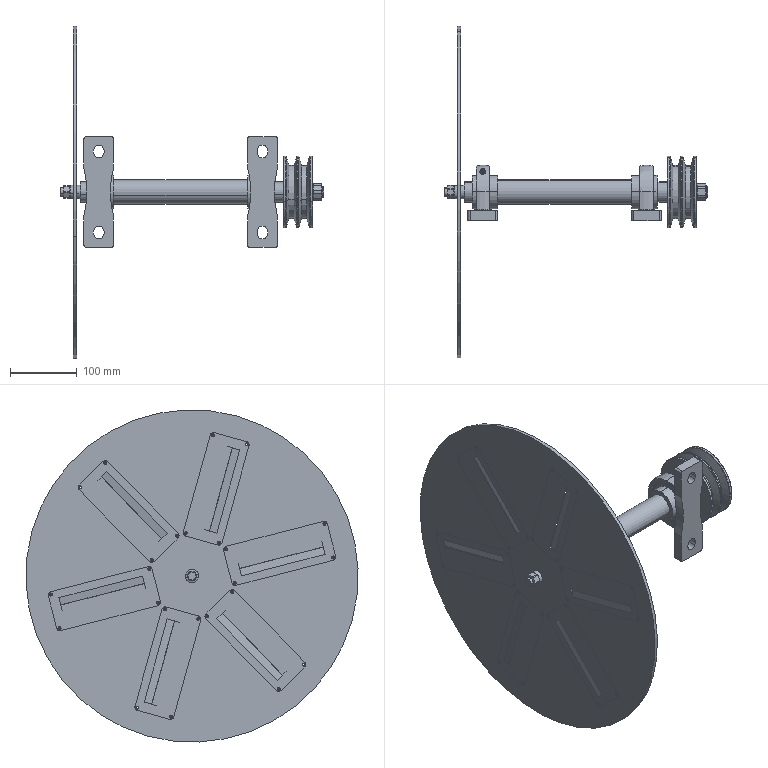Part | SolidWorks | features ReferencePattern 5, LocalCirPattern 1 | 21 solids | 677 faces | box 394 x 496 x 496 mm | volume 1816231 mm3 | cylinder 326 | plane 242 | cone 87 | spline 22 | commonest cylinder face diameters 2.4 x96 10 x82 20 x15 16 x14 2 x12 14 x10